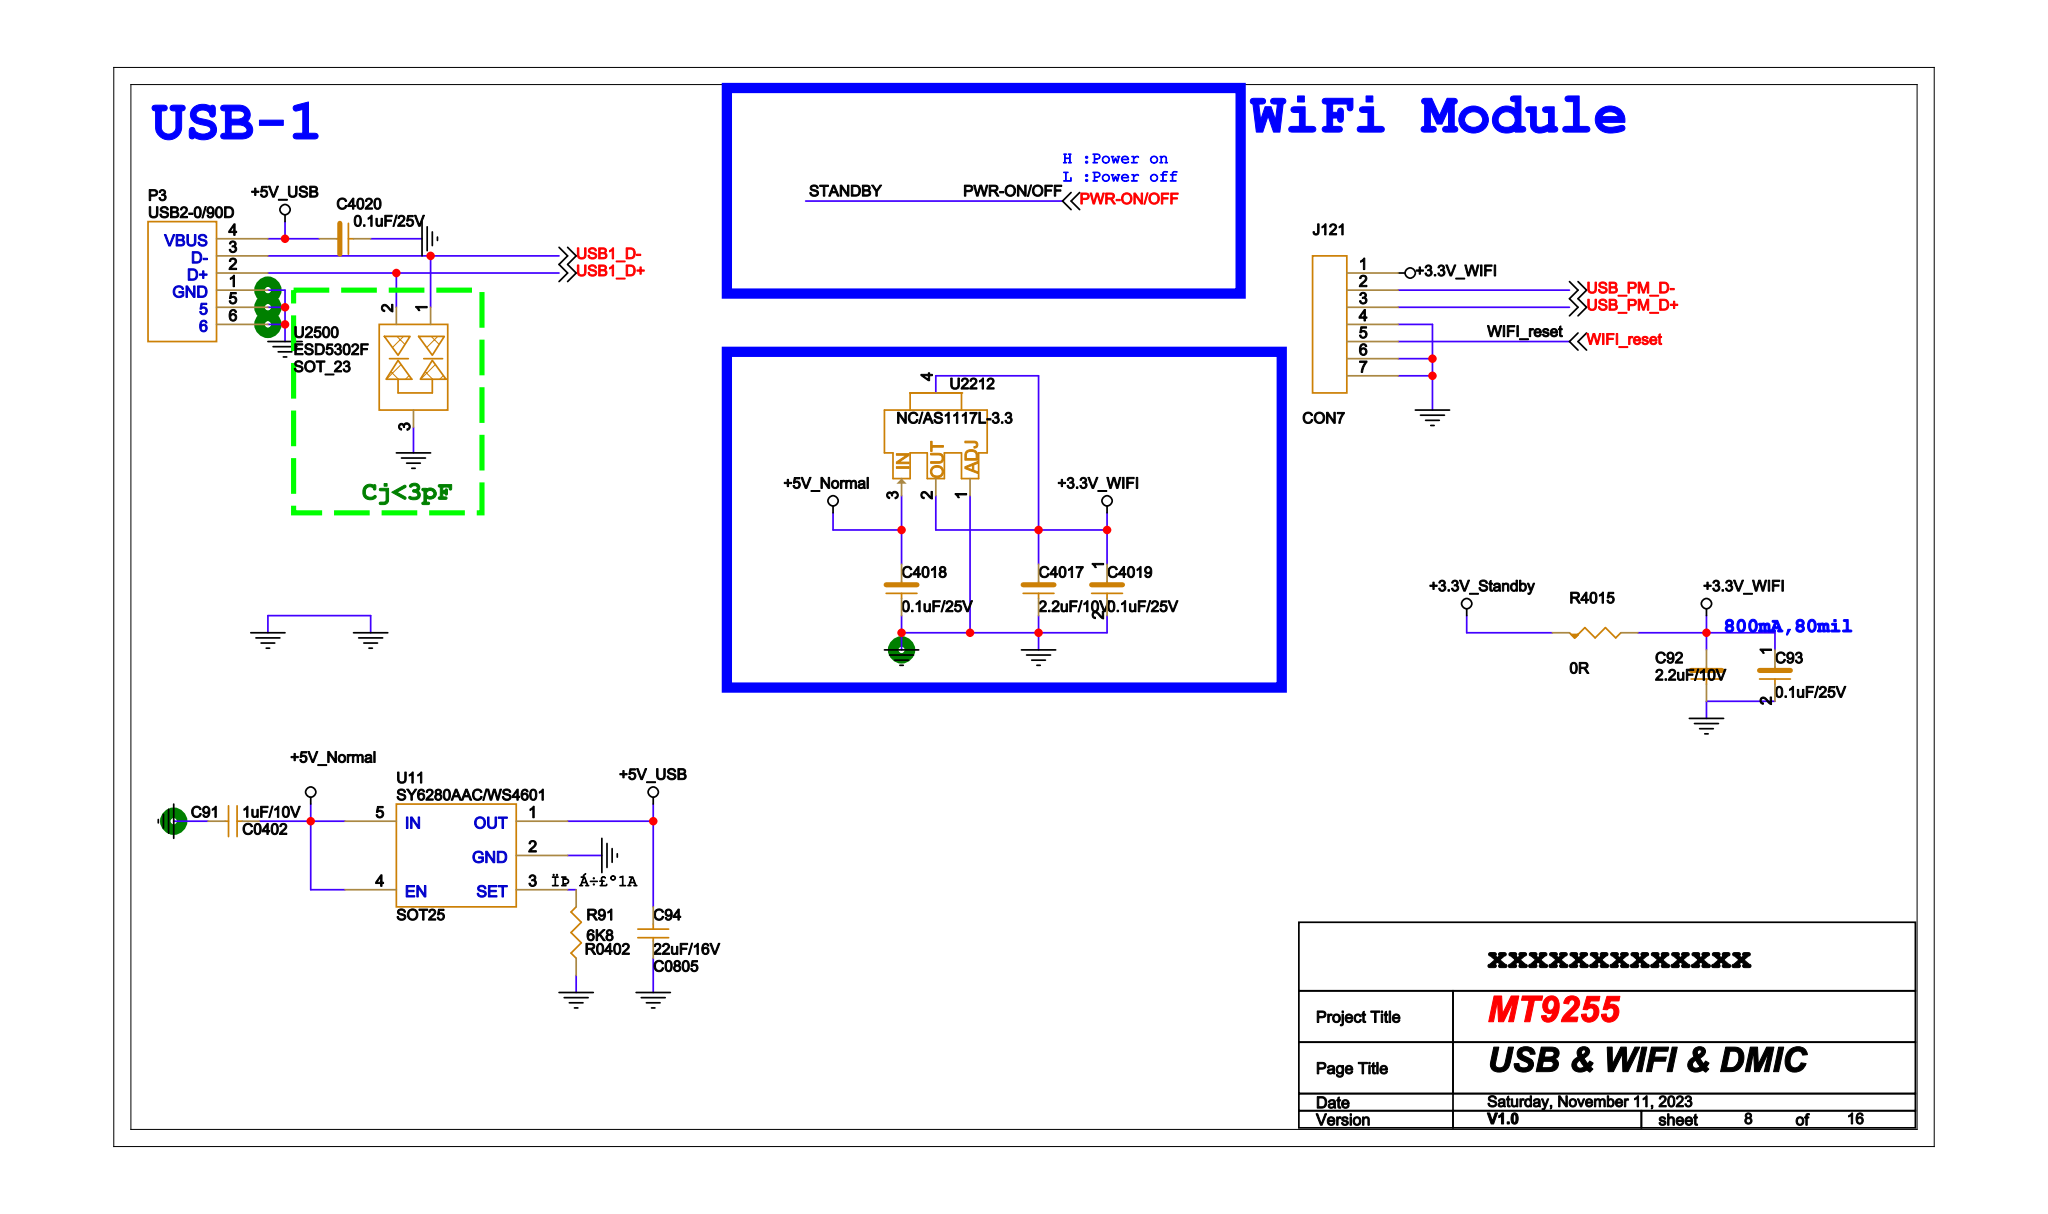Circuit board | Cadence Allegro | 1223 parts | 777 nets | one sheet of the schematic
Parts on this sheet (reference | value | footprint):
C91 | 1uF/10V | C0402
C92 | 2.2uF/10V | C0402
C93 | 0.1uF/25V | C0402
C94 | 22uF/16V | C0805
C4017 | 2.2uF/10V | C0402
C4018 | 0.1uF/25V | C0402
C4019 | 0.1uF/25V | C0402
C4020 | 0.1uF/25V | C0402
J121 | CON7 | CN1X5-1P25MM-WF
P3 | USB2-0/90D | USB-164P
R91 | 6K8 | R0402
R4015 | 0R | R0603
U11 | SY6280AAC/WS4601 | SOT25
U2212 | NC/AS1117L-3.3 | SOT-223
U2500 | ESD5302F | SOT_23
Nets of these parts (net: part-pin ...):
GND: C91-1 C92-2 C93-2 C94-1 C4017-2 C4018-2 C4019-2 C4020-2 J121-4 J121-6 J121-7 P3-1 P3-5 P3-6 R91-1 U11-2 U2212-1 U2500-3
+3.3V_STANDBY: R4015-1
+5V_NORMAL: C91-2 C4018-1 U11-4 U11-5 U2212-3
+3.3V_WIFI: C92-1 C93-1 C4017-1 C4019-1 J121-1 R4015-2 U2212-2 U2212-4
+5V_USB: C94-2 C4020-1 P3-4 U11-1
USB_PM_D-: J121-2
USB_PM_D+: J121-3
WIFI_RESET: J121-5
USB1_D+: P3-2 U2500-2
USB1_D-: P3-3 U2500-1
N24198869: R91-2 U11-3